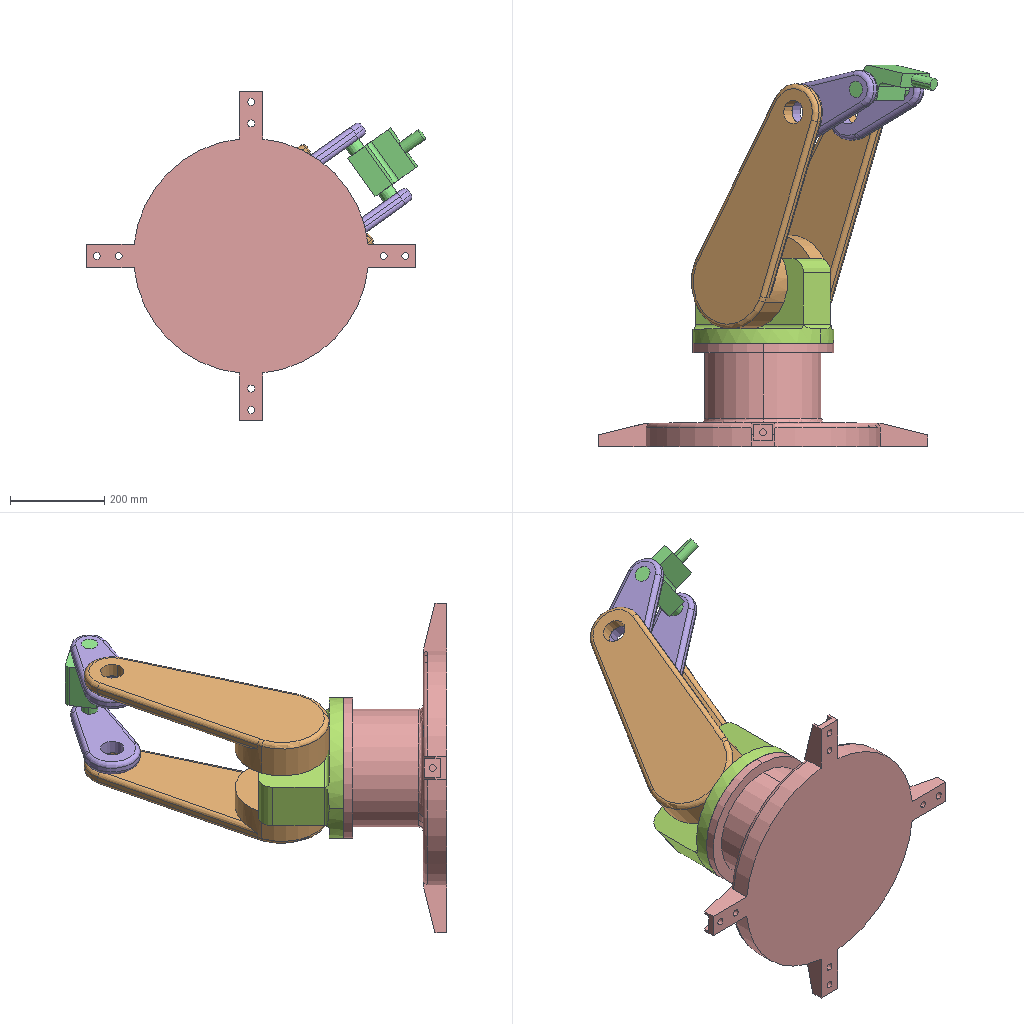Assembly | SolidWorks | 6 different items | 8 placed | box 721 x 811 x 700 mm
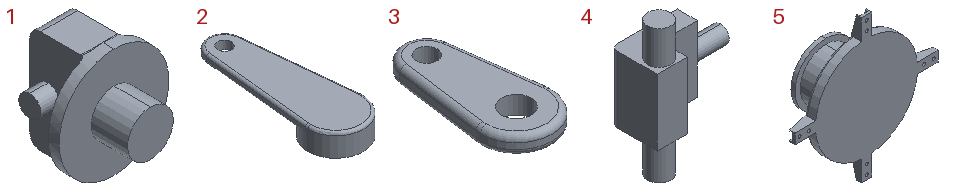Parts list (item | name | quantity | size | volume | features):
1 | - | x1 | 300 x 280 x 300 mm | 7882331 mm3 | features Revolution 3, ICE 2, BaseBody 1, Fillet 1
2 | - | x2 | 200 x 560.023 x 80 mm | 3893750 mm3 | features HoleWzd 2, Extrusion 1, Fillet 1, ICE 1
3 | - | x2 | 120 x 250 x 30 mm | 585410 mm3 | features HoleWzd 2, Extrusion 1, Fillet 1
4 | - | x1 | 150 x 70 x 200.87 mm | 603595 mm3 | features Revolution 3, Extrusion 1, Fillet 1, ICE 1
5 | - | x1 | 700 x 220 x 700 mm | 17727332 mm3 | features HoleWzd 6, ICE 5, BaseBody 1, Fillet 1, Revolution 1
6 | hanger 2 | x1 | - | - | -